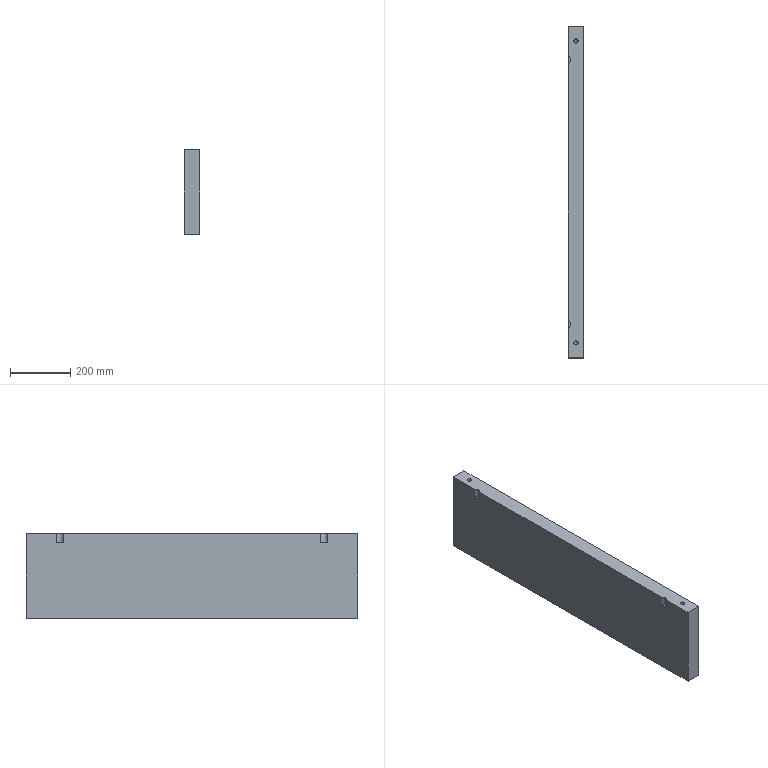Part | NX | features 29 2 | 1 solid | 20 faces | box 50 x 1105 x 280.5 mm | volume 15459680 mm3 | plane 8 | cylinder 7 | cone 5 | commonest cylinder face diameters 14.1 x5 28 x2
STEP:
#1=CARTESIAN_POINT('',(2006.023,-502.5,-493.5));
#2=VERTEX_POINT('',#1);
#3=CARTESIAN_POINT('',(1998.973,-502.5,-493.5));
#4=DIRECTION('',(0.,0.,1.));
#5=DIRECTION('',(1.,0.,0.));
#6=AXIS2_PLACEMENT_3D('',#3,#4,#5);
#7=CIRCLE('',#6,7.05);
#8=EDGE_CURVE('',#2,#2,#7,.T.);
#9=ORIENTED_EDGE('',*,*,#8,.T.);
#10=EDGE_LOOP('',(#9));
#11=FACE_BOUND('',#10,.T.);
#12=CARTESIAN_POINT('',(1973.973,552.5,-493.5));
#13=VERTEX_POINT('',#12);
#14=CARTESIAN_POINT('',(1973.973,-552.5,-493.5));
#15=VERTEX_POINT('',#14);
#16=CARTESIAN_POINT('',(1973.973,193.,-493.5));
#17=DIRECTION('',(0.,-1.,0.));
#18=VECTOR('',#17,1000.);
#19=LINE('',#16,#18);
#20=EDGE_CURVE('',#13,#15,#19,.T.);
#21=ORIENTED_EDGE('',*,*,#20,.F.);
#22=CARTESIAN_POINT('',(2023.973,552.5,-493.5));
#23=VERTEX_POINT('',#22);
#24=CARTESIAN_POINT('',(2773.973,552.5,-493.5));
#25=DIRECTION('',(1.,0.,0.));
#26=VECTOR('',#25,1000.);
#27=LINE('',#24,#26);
#28=EDGE_CURVE('',#13,#23,#27,.T.);
#29=ORIENTED_EDGE('',*,*,#28,.T.);
#30=CARTESIAN_POINT('',(2023.973,-552.5,-493.5));
#31=VERTEX_POINT('',#30);
#32=CARTESIAN_POINT('',(2023.973,193.,-493.5));
#33=DIRECTION('',(0.,1.,0.));
#34=VECTOR('',#33,1000.);
#35=LINE('',#32,#34);
#36=EDGE_CURVE('',#31,#23,#35,.T.);
#37=ORIENTED_EDGE('',*,*,#36,.F.);
#38=CARTESIAN_POINT('',(2773.973,-552.5,-493.5));
#39=DIRECTION('',(-1.,0.,0.));
#40=VECTOR('',#39,1000.);
#41=LINE('',#38,#40);
#42=EDGE_CURVE('',#31,#15,#41,.T.);
#43=ORIENTED_EDGE('',*,*,#42,.T.);
#44=EDGE_LOOP('',(#21,#29,#37,#43));
#45=FACE_BOUND('',#44,.T.);
#46=CARTESIAN_POINT('',(2006.023,502.5,-493.5));
#47=VERTEX_POINT('',#46);
#48=CARTESIAN_POINT('',(1998.973,502.5,-493.5));
#49=DIRECTION('',(0.,0.,1.));
#50=DIRECTION('',(1.,0.,0.));
#51=AXIS2_PLACEMENT_3D('',#48,#49,#50);
#52=CIRCLE('',#51,7.05);
#53=EDGE_CURVE('',#47,#47,#52,.T.);
#54=ORIENTED_EDGE('',*,*,#53,.T.);
#55=EDGE_LOOP('',(#54));
#56=FACE_BOUND('',#55,.T.);
#57=CARTESIAN_POINT('',(2006.023,0.,-493.5));
#58=VERTEX_POINT('',#57);
#59=CARTESIAN_POINT('',(1998.973,0.,-493.5));
#60=DIRECTION('',(0.,0.,1.));
#61=DIRECTION('',(1.,0.,0.));
#62=AXIS2_PLACEMENT_3D('',#59,#60,#61);
#63=CIRCLE('',#62,7.05);
#64=EDGE_CURVE('',#58,#58,#63,.T.);
#65=ORIENTED_EDGE('',*,*,#64,.T.);
#66=EDGE_LOOP('',(#65));
#67=FACE_BOUND('',#66,.T.);
#68=CARTESIAN_POINT('',(2773.973,0.,-493.5));
#69=DIRECTION('',(0.,0.,-1.));
#70=DIRECTION('',(1.,0.,0.));
#71=AXIS2_PLACEMENT_3D('',#68,#69,#70);
#72=PLANE('',#71);
#73=ADVANCED_FACE('',(#11,#45,#56,#67),#72,.T.);
#74=CARTESIAN_POINT('',(2006.023,-502.5,-213.));
#75=VERTEX_POINT('',#74);
#76=CARTESIAN_POINT('',(1998.973,-502.5,-213.));
#77=DIRECTION('',(0.,0.,-1.));
#78=DIRECTION('',(1.,0.,0.));
#79=AXIS2_PLACEMENT_3D('',#76,#77,#78);
#80=CIRCLE('',#79,7.05);
#81=EDGE_CURVE('',#75,#75,#80,.T.);
#82=ORIENTED_EDGE('',*,*,#81,.T.);
#83=EDGE_LOOP('',(#82));
#84=FACE_BOUND('',#83,.T.);
#85=CARTESIAN_POINT('',(1973.973,427.86,-213.));
#86=VERTEX_POINT('',#85);
#87=CARTESIAN_POINT('',(1973.973,452.14,-213.));
#88=VERTEX_POINT('',#87);
#89=CARTESIAN_POINT('',(1967.,440.,-213.));
#90=DIRECTION('',(0.,0.,1.));
#91=DIRECTION('',(-1.,0.,0.));
#92=AXIS2_PLACEMENT_3D('',#89,#90,#91);
#93=CIRCLE('',#92,14.);
#94=EDGE_CURVE('',#86,#88,#93,.T.);
#95=ORIENTED_EDGE('',*,*,#94,.F.);
#96=CARTESIAN_POINT('',(1973.973,-427.86,-213.));
#97=VERTEX_POINT('',#96);
#98=CARTESIAN_POINT('',(1973.973,193.,-213.));
#99=DIRECTION('',(0.,1.,0.));
#100=VECTOR('',#99,1000.);
#101=LINE('',#98,#100);
#102=EDGE_CURVE('',#97,#86,#101,.T.);
#103=ORIENTED_EDGE('',*,*,#102,.F.);
#104=CARTESIAN_POINT('',(1973.973,-452.14,-213.));
#105=VERTEX_POINT('',#104);
#106=CARTESIAN_POINT('',(1967.,-440.,-213.));
#107=DIRECTION('',(0.,0.,-1.));
#108=DIRECTION('',(-1.,0.,0.));
#109=AXIS2_PLACEMENT_3D('',#106,#107,#108);
#110=CIRCLE('',#109,14.);
#111=EDGE_CURVE('',#97,#105,#110,.T.);
#112=ORIENTED_EDGE('',*,*,#111,.T.);
#113=CARTESIAN_POINT('',(1973.973,-552.5,-213.));
#114=VERTEX_POINT('',#113);
#115=CARTESIAN_POINT('',(1973.973,193.,-213.));
#116=DIRECTION('',(0.,1.,0.));
#117=VECTOR('',#116,1000.);
#118=LINE('',#115,#117);
#119=EDGE_CURVE('',#114,#105,#118,.T.);
#120=ORIENTED_EDGE('',*,*,#119,.F.);
#121=CARTESIAN_POINT('',(2023.973,-552.5,-213.));
#122=VERTEX_POINT('',#121);
#123=CARTESIAN_POINT('',(2773.973,-552.5,-213.));
#124=DIRECTION('',(1.,0.,0.));
#125=VECTOR('',#124,1000.);
#126=LINE('',#123,#125);
#127=EDGE_CURVE('',#114,#122,#126,.T.);
#128=ORIENTED_EDGE('',*,*,#127,.T.);
#129=CARTESIAN_POINT('',(2023.973,552.5,-213.));
#130=VERTEX_POINT('',#129);
#131=CARTESIAN_POINT('',(2023.973,193.,-213.));
#132=DIRECTION('',(0.,-1.,0.));
#133=VECTOR('',#132,1000.);
#134=LINE('',#131,#133);
#135=EDGE_CURVE('',#130,#122,#134,.T.);
#136=ORIENTED_EDGE('',*,*,#135,.F.);
#137=CARTESIAN_POINT('',(1973.973,552.5,-213.));
#138=VERTEX_POINT('',#137);
#139=CARTESIAN_POINT('',(2773.973,552.5,-213.));
#140=DIRECTION('',(-1.,0.,0.));
#141=VECTOR('',#140,1000.);
#142=LINE('',#139,#141);
#143=EDGE_CURVE('',#130,#138,#142,.T.);
#144=ORIENTED_EDGE('',*,*,#143,.T.);
#145=CARTESIAN_POINT('',(1973.973,193.,-213.));
#146=DIRECTION('',(0.,1.,0.));
#147=VECTOR('',#146,1000.);
#148=LINE('',#145,#147);
#149=EDGE_CURVE('',#88,#138,#148,.T.);
#150=ORIENTED_EDGE('',*,*,#149,.F.);
#151=EDGE_LOOP('',(#95,#103,#112,#120,#128,#136,#144,#150));
#152=FACE_BOUND('',#151,.T.);
#153=CARTESIAN_POINT('',(2006.023,502.5,-213.));
#154=VERTEX_POINT('',#153);
#155=CARTESIAN_POINT('',(1998.973,502.5,-213.));
#156=DIRECTION('',(0.,0.,-1.));
#157=DIRECTION('',(1.,0.,0.));
#158=AXIS2_PLACEMENT_3D('',#155,#156,#157);
#159=CIRCLE('',#158,7.05);
#160=EDGE_CURVE('',#154,#154,#159,.T.);
#161=ORIENTED_EDGE('',*,*,#160,.T.);
#162=EDGE_LOOP('',(#161));
#163=FACE_BOUND('',#162,.T.);
#164=CARTESIAN_POINT('',(2773.973,0.,-213.));
#165=DIRECTION('',(0.,0.,1.));
#166=DIRECTION('',(-1.,0.,0.));
#167=AXIS2_PLACEMENT_3D('',#164,#165,#166);
#168=PLANE('',#167);
#169=ADVANCED_FACE('',(#84,#152,#163),#168,.T.);
#170=CARTESIAN_POINT('',(1973.973,427.86,-243.));
#171=VERTEX_POINT('',#170);
#172=CARTESIAN_POINT('',(1973.973,427.86,-243.));
#173=DIRECTION('',(0.,0.,1.));
#174=VECTOR('',#173,1000.);
#175=LINE('',#172,#174);
#176=EDGE_CURVE('',#171,#86,#175,.T.);
#177=ORIENTED_EDGE('',*,*,#176,.F.);
#178=CARTESIAN_POINT('',(1973.973,452.14,-243.));
#179=VERTEX_POINT('',#178);
#180=CARTESIAN_POINT('',(1973.973,193.,-243.));
#181=DIRECTION('',(0.,1.,0.));
#182=VECTOR('',#181,1000.);
#183=LINE('',#180,#182);
#184=EDGE_CURVE('',#171,#179,#183,.T.);
#185=ORIENTED_EDGE('',*,*,#184,.T.);
#186=CARTESIAN_POINT('',(1973.973,452.14,-243.));
#187=DIRECTION('',(0.,0.,-1.));
#188=VECTOR('',#187,1000.);
#189=LINE('',#186,#188);
#190=EDGE_CURVE('',#88,#179,#189,.T.);
#191=ORIENTED_EDGE('',*,*,#190,.F.);
#192=ORIENTED_EDGE('',*,*,#149,.T.);
#193=CARTESIAN_POINT('',(1973.973,552.5,-205.5));
#194=DIRECTION('',(0.,0.,-1.));
#195=VECTOR('',#194,1000.);
#196=LINE('',#193,#195);
#197=EDGE_CURVE('',#138,#13,#196,.T.);
#198=ORIENTED_EDGE('',*,*,#197,.T.);
#199=ORIENTED_EDGE('',*,*,#20,.T.);
#200=CARTESIAN_POINT('',(1973.973,-552.5,-205.5));
#201=DIRECTION('',(0.,0.,1.));
#202=VECTOR('',#201,1000.);
#203=LINE('',#200,#202);
#204=EDGE_CURVE('',#15,#114,#203,.T.);
#205=ORIENTED_EDGE('',*,*,#204,.T.);
#206=ORIENTED_EDGE('',*,*,#119,.T.);
#207=CARTESIAN_POINT('',(1973.973,-452.14,-243.));
#208=VERTEX_POINT('',#207);
#209=CARTESIAN_POINT('',(1973.973,-452.14,-243.));
#210=DIRECTION('',(0.,0.,-1.));
#211=VECTOR('',#210,1000.);
#212=LINE('',#209,#211);
#213=EDGE_CURVE('',#105,#208,#212,.T.);
#214=ORIENTED_EDGE('',*,*,#213,.T.);
#215=CARTESIAN_POINT('',(1973.973,-427.86,-243.));
#216=VERTEX_POINT('',#215);
#217=CARTESIAN_POINT('',(1973.973,193.,-243.));
#218=DIRECTION('',(0.,-1.,0.));
#219=VECTOR('',#218,1000.);
#220=LINE('',#217,#219);
#221=EDGE_CURVE('',#216,#208,#220,.T.);
#222=ORIENTED_EDGE('',*,*,#221,.F.);
#223=CARTESIAN_POINT('',(1973.973,-427.86,-243.));
#224=DIRECTION('',(0.,0.,1.));
#225=VECTOR('',#224,1000.);
#226=LINE('',#223,#225);
#227=EDGE_CURVE('',#216,#97,#226,.T.);
#228=ORIENTED_EDGE('',*,*,#227,.T.);
#229=ORIENTED_EDGE('',*,*,#102,.T.);
#230=EDGE_LOOP('',(#177,#185,#191,#192,#198,#199,#205,#206,#214,#222,#228,#229));
#231=FACE_BOUND('',#230,.T.);
#232=CARTESIAN_POINT('',(1973.973,193.,-205.5));
#233=DIRECTION('',(-1.,0.,0.));
#234=DIRECTION('',(0.,0.,1.));
#235=AXIS2_PLACEMENT_3D('',#232,#233,#234);
#236=PLANE('',#235);
#237=ADVANCED_FACE('',(#231),#236,.T.);
#238=ORIENTED_EDGE('',*,*,#143,.F.);
#239=CARTESIAN_POINT('',(2023.973,552.5,-205.5));
#240=DIRECTION('',(0.,0.,1.));
#241=VECTOR('',#240,1000.);
#242=LINE('',#239,#241);
#243=EDGE_CURVE('',#23,#130,#242,.T.);
#244=ORIENTED_EDGE('',*,*,#243,.F.);
#245=ORIENTED_EDGE('',*,*,#28,.F.);
#246=ORIENTED_EDGE('',*,*,#197,.F.);
#247=EDGE_LOOP('',(#238,#244,#245,#246));
#248=FACE_BOUND('',#247,.T.);
#249=CARTESIAN_POINT('',(282.5,552.5,91.));
#250=DIRECTION('',(0.,-1.,0.));
#251=DIRECTION('',(-1.,0.,0.));
#252=AXIS2_PLACEMENT_3D('',#249,#250,#251);
#253=PLANE('',#252);
#254=ADVANCED_FACE('',(#248),#253,.F.);
#255=ORIENTED_EDGE('',*,*,#36,.T.);
#256=ORIENTED_EDGE('',*,*,#243,.T.);
#257=ORIENTED_EDGE('',*,*,#135,.T.);
#258=CARTESIAN_POINT('',(2023.973,-552.5,-205.5));
#259=DIRECTION('',(0.,0.,-1.));
#260=VECTOR('',#259,1000.);
#261=LINE('',#258,#260);
#262=EDGE_CURVE('',#122,#31,#261,.T.);
#263=ORIENTED_EDGE('',*,*,#262,.T.);
#264=EDGE_LOOP('',(#255,#256,#257,#263));
#265=FACE_BOUND('',#264,.T.);
#266=CARTESIAN_POINT('',(2023.973,193.,-205.5));
#267=DIRECTION('',(1.,0.,0.));
#268=DIRECTION('',(0.,0.,-1.));
#269=AXIS2_PLACEMENT_3D('',#266,#267,#268);
#270=PLANE('',#269);
#271=ADVANCED_FACE('',(#265),#270,.T.);
#272=ORIENTED_EDGE('',*,*,#127,.F.);
#273=ORIENTED_EDGE('',*,*,#204,.F.);
#274=ORIENTED_EDGE('',*,*,#42,.F.);
#275=ORIENTED_EDGE('',*,*,#262,.F.);
#276=EDGE_LOOP('',(#272,#273,#274,#275));
#277=FACE_BOUND('',#276,.T.);
#278=CARTESIAN_POINT('',(282.5,-552.5,-113.));
#279=DIRECTION('',(0.,1.,0.));
#280=DIRECTION('',(1.,0.,0.));
#281=AXIS2_PLACEMENT_3D('',#278,#279,#280);
#282=PLANE('',#281);
#283=ADVANCED_FACE('',(#277),#282,.F.);
#284=ORIENTED_EDGE('',*,*,#111,.F.);
#285=ORIENTED_EDGE('',*,*,#227,.F.);
#286=CARTESIAN_POINT('',(1967.,-440.,-243.));
#287=DIRECTION('',(0.,0.,1.));
#288=DIRECTION('',(-1.,0.,0.));
#289=AXIS2_PLACEMENT_3D('',#286,#287,#288);
#290=CIRCLE('',#289,14.);
#291=EDGE_CURVE('',#208,#216,#290,.T.);
#292=ORIENTED_EDGE('',*,*,#291,.F.);
#293=ORIENTED_EDGE('',*,*,#213,.F.);
#294=EDGE_LOOP('',(#284,#285,#292,#293));
#295=FACE_BOUND('',#294,.T.);
#296=CARTESIAN_POINT('',(1967.,-440.,-243.));
#297=DIRECTION('',(0.,0.,1.));
#298=DIRECTION('',(-1.,0.,0.));
#299=AXIS2_PLACEMENT_3D('',#296,#297,#298);
#300=CYLINDRICAL_SURFACE('',#299,14.);
#301=ADVANCED_FACE('',(#295),#300,.F.);
#302=ORIENTED_EDGE('',*,*,#221,.T.);
#303=ORIENTED_EDGE('',*,*,#291,.T.);
#304=EDGE_LOOP('',(#302,#303));
#305=FACE_BOUND('',#304,.T.);
#306=CARTESIAN_POINT('',(1967.,-440.,-243.));
#307=DIRECTION('',(0.,0.,-1.));
#308=DIRECTION('',(1.,0.,0.));
#309=AXIS2_PLACEMENT_3D('',#306,#307,#308);
#310=PLANE('',#309);
#311=ADVANCED_FACE('',(#305),#310,.F.);
#312=ORIENTED_EDGE('',*,*,#176,.T.);
#313=ORIENTED_EDGE('',*,*,#94,.T.);
#314=ORIENTED_EDGE('',*,*,#190,.T.);
#315=CARTESIAN_POINT('',(1967.,440.,-243.));
#316=DIRECTION('',(0.,0.,-1.));
#317=DIRECTION('',(-1.,0.,0.));
#318=AXIS2_PLACEMENT_3D('',#315,#316,#317);
#319=CIRCLE('',#318,14.);
#320=EDGE_CURVE('',#179,#171,#319,.T.);
#321=ORIENTED_EDGE('',*,*,#320,.T.);
#322=EDGE_LOOP('',(#312,#313,#314,#321));
#323=FACE_BOUND('',#322,.T.);
#324=CARTESIAN_POINT('',(1967.,440.,-243.));
#325=DIRECTION('',(0.,0.,1.));
#326=DIRECTION('',(-1.,0.,0.));
#327=AXIS2_PLACEMENT_3D('',#324,#325,#326);
#328=CYLINDRICAL_SURFACE('',#327,14.);
#329=ADVANCED_FACE('',(#323),#328,.F.);
#330=ORIENTED_EDGE('',*,*,#320,.F.);
#331=ORIENTED_EDGE('',*,*,#184,.F.);
#332=EDGE_LOOP('',(#330,#331));
#333=FACE_BOUND('',#332,.T.);
#334=CARTESIAN_POINT('',(1967.,440.,-243.));
#335=DIRECTION('',(0.,0.,1.));
#336=DIRECTION('',(-1.,0.,0.));
#337=AXIS2_PLACEMENT_3D('',#334,#335,#336);
#338=PLANE('',#337);
#339=ADVANCED_FACE('',(#333),#338,.T.);
#340=CARTESIAN_POINT('',(1991.923,-502.5,-249.95));
#341=VERTEX_POINT('',#340);
#342=CARTESIAN_POINT('',(1998.973,-502.5,-249.95));
#343=DIRECTION('',(0.,0.,-1.));
#344=DIRECTION('',(-1.,0.,0.));
#345=AXIS2_PLACEMENT_3D('',#342,#343,#344);
#346=CIRCLE('',#345,7.05);
#347=EDGE_CURVE('',#341,#341,#346,.T.);
#348=ORIENTED_EDGE('',*,*,#347,.T.);
#349=EDGE_LOOP('',(#348));
#350=FACE_BOUND('',#349,.T.);
#351=ORIENTED_EDGE('',*,*,#81,.F.);
#352=EDGE_LOOP('',(#351));
#353=FACE_BOUND('',#352,.T.);
#354=CARTESIAN_POINT('',(1998.973,-502.5,-213.));
#355=DIRECTION('',(0.,0.,-1.));
#356=DIRECTION('',(-1.,0.,0.));
#357=AXIS2_PLACEMENT_3D('',#354,#355,#356);
#358=CYLINDRICAL_SURFACE('',#357,7.05);
#359=ADVANCED_FACE('',(#350,#353),#358,.F.);
#360=CARTESIAN_POINT('',(1998.973,-502.5,-257.));
#361=VERTEX_POINT('',#360);
#362=VERTEX_LOOP('',#361);
#363=FACE_BOUND('',#362,.T.);
#364=ORIENTED_EDGE('',*,*,#347,.F.);
#365=EDGE_LOOP('',(#364));
#366=FACE_BOUND('',#365,.T.);
#367=CARTESIAN_POINT('',(1998.973,-502.5,-249.95));
#368=DIRECTION('',(0.,0.,1.));
#369=DIRECTION('',(-1.,0.,0.));
#370=AXIS2_PLACEMENT_3D('',#367,#368,#369);
#371=CONICAL_SURFACE('',#370,7.05,0.7854);
#372=ADVANCED_FACE('',(#363,#366),#371,.F.);
#373=CARTESIAN_POINT('',(1991.923,502.5,-249.95));
#374=VERTEX_POINT('',#373);
#375=CARTESIAN_POINT('',(1998.973,502.5,-249.95));
#376=DIRECTION('',(0.,0.,-1.));
#377=DIRECTION('',(-1.,0.,0.));
#378=AXIS2_PLACEMENT_3D('',#375,#376,#377);
#379=CIRCLE('',#378,7.05);
#380=EDGE_CURVE('',#374,#374,#379,.T.);
#381=ORIENTED_EDGE('',*,*,#380,.T.);
#382=EDGE_LOOP('',(#381));
#383=FACE_BOUND('',#382,.T.);
#384=ORIENTED_EDGE('',*,*,#160,.F.);
#385=EDGE_LOOP('',(#384));
#386=FACE_BOUND('',#385,.T.);
#387=CARTESIAN_POINT('',(1998.973,502.5,-213.));
#388=DIRECTION('',(0.,0.,-1.));
#389=DIRECTION('',(-1.,0.,0.));
#390=AXIS2_PLACEMENT_3D('',#387,#388,#389);
#391=CYLINDRICAL_SURFACE('',#390,7.05);
#392=ADVANCED_FACE('',(#383,#386),#391,.F.);
#393=CARTESIAN_POINT('',(1998.973,502.5,-257.));
#394=VERTEX_POINT('',#393);
#395=VERTEX_LOOP('',#394);
#396=FACE_BOUND('',#395,.T.);
#397=ORIENTED_EDGE('',*,*,#380,.F.);
#398=EDGE_LOOP('',(#397));
#399=FACE_BOUND('',#398,.T.);
#400=CARTESIAN_POINT('',(1998.973,502.5,-249.95));
#401=DIRECTION('',(0.,0.,1.));
#402=DIRECTION('',(-1.,0.,0.));
#403=AXIS2_PLACEMENT_3D('',#400,#401,#402);
#404=CONICAL_SURFACE('',#403,7.05,0.7854);
#405=ADVANCED_FACE('',(#396,#399),#404,.F.);
#406=CARTESIAN_POINT('',(2006.023,502.5,-456.55));
#407=VERTEX_POINT('',#406);
#408=CARTESIAN_POINT('',(1998.973,502.5,-456.55));
#409=DIRECTION('',(0.,0.,1.));
#410=DIRECTION('',(1.,0.,0.));
#411=AXIS2_PLACEMENT_3D('',#408,#409,#410);
#412=CIRCLE('',#411,7.05);
#413=EDGE_CURVE('',#407,#407,#412,.T.);
#414=ORIENTED_EDGE('',*,*,#413,.T.);
#415=EDGE_LOOP('',(#414));
#416=FACE_BOUND('',#415,.T.);
#417=ORIENTED_EDGE('',*,*,#53,.F.);
#418=EDGE_LOOP('',(#417));
#419=FACE_BOUND('',#418,.T.);
#420=CARTESIAN_POINT('',(1998.973,502.5,-493.5));
#421=DIRECTION('',(0.,0.,1.));
#422=DIRECTION('',(-1.,0.,0.));
#423=AXIS2_PLACEMENT_3D('',#420,#421,#422);
#424=CYLINDRICAL_SURFACE('',#423,7.05);
#425=ADVANCED_FACE('',(#416,#419),#424,.F.);
#426=CARTESIAN_POINT('',(1998.973,502.5,-449.5));
#427=VERTEX_POINT('',#426);
#428=VERTEX_LOOP('',#427);
#429=FACE_BOUND('',#428,.T.);
#430=ORIENTED_EDGE('',*,*,#413,.F.);
#431=EDGE_LOOP('',(#430));
#432=FACE_BOUND('',#431,.T.);
#433=CARTESIAN_POINT('',(1998.973,502.5,-456.55));
#434=DIRECTION('',(0.,0.,-1.));
#435=DIRECTION('',(1.,0.,0.));
#436=AXIS2_PLACEMENT_3D('',#433,#434,#435);
#437=CONICAL_SURFACE('',#436,7.05,0.7854);
#438=ADVANCED_FACE('',(#429,#432),#437,.F.);
#439=CARTESIAN_POINT('',(2006.023,-502.5,-456.55));
#440=VERTEX_POINT('',#439);
#441=CARTESIAN_POINT('',(1998.973,-502.5,-456.55));
#442=DIRECTION('',(0.,0.,1.));
#443=DIRECTION('',(1.,0.,0.));
#444=AXIS2_PLACEMENT_3D('',#441,#442,#443);
#445=CIRCLE('',#444,7.05);
#446=EDGE_CURVE('',#440,#440,#445,.T.);
#447=ORIENTED_EDGE('',*,*,#446,.T.);
#448=EDGE_LOOP('',(#447));
#449=FACE_BOUND('',#448,.T.);
#450=ORIENTED_EDGE('',*,*,#8,.F.);
#451=EDGE_LOOP('',(#450));
#452=FACE_BOUND('',#451,.T.);
#453=CARTESIAN_POINT('',(1998.973,-502.5,-493.5));
#454=DIRECTION('',(0.,0.,1.));
#455=DIRECTION('',(-1.,0.,0.));
#456=AXIS2_PLACEMENT_3D('',#453,#454,#455);
#457=CYLINDRICAL_SURFACE('',#456,7.05);
#458=ADVANCED_FACE('',(#449,#452),#457,.F.);
#459=CARTESIAN_POINT('',(1998.973,-502.5,-449.5));
#460=VERTEX_POINT('',#459);
#461=VERTEX_LOOP('',#460);
#462=FACE_BOUND('',#461,.T.);
#463=ORIENTED_EDGE('',*,*,#446,.F.);
#464=EDGE_LOOP('',(#463));
#465=FACE_BOUND('',#464,.T.);
#466=CARTESIAN_POINT('',(1998.973,-502.5,-456.55));
#467=DIRECTION('',(0.,0.,-1.));
#468=DIRECTION('',(1.,0.,0.));
#469=AXIS2_PLACEMENT_3D('',#466,#467,#468);
#470=CONICAL_SURFACE('',#469,7.05,0.7854);
#471=ADVANCED_FACE('',(#462,#465),#470,.F.);
#472=CARTESIAN_POINT('',(2006.023,0.,-456.55));
#473=VERTEX_POINT('',#472);
#474=CARTESIAN_POINT('',(1998.973,0.,-456.55));
#475=DIRECTION('',(0.,0.,1.));
#476=DIRECTION('',(1.,0.,0.));
#477=AXIS2_PLACEMENT_3D('',#474,#475,#476);
#478=CIRCLE('',#477,7.05);
#479=EDGE_CURVE('',#473,#473,#478,.T.);
#480=ORIENTED_EDGE('',*,*,#479,.T.);
#481=EDGE_LOOP('',(#480));
#482=FACE_BOUND('',#481,.T.);
#483=ORIENTED_EDGE('',*,*,#64,.F.);
#484=EDGE_LOOP('',(#483));
#485=FACE_BOUND('',#484,.T.);
#486=CARTESIAN_POINT('',(1998.973,0.,-493.5));
#487=DIRECTION('',(0.,0.,1.));
#488=DIRECTION('',(-1.,0.,0.));
#489=AXIS2_PLACEMENT_3D('',#486,#487,#488);
#490=CYLINDRICAL_SURFACE('',#489,7.05);
#491=ADVANCED_FACE('',(#482,#485),#490,.F.);
#492=CARTESIAN_POINT('',(1998.973,0.,-449.5));
#493=VERTEX_POINT('',#492);
#494=VERTEX_LOOP('',#493);
#495=FACE_BOUND('',#494,.T.);
#496=ORIENTED_EDGE('',*,*,#479,.F.);
#497=EDGE_LOOP('',(#496));
#498=FACE_BOUND('',#497,.T.);
#499=CARTESIAN_POINT('',(1998.973,0.,-456.55));
#500=DIRECTION('',(0.,0.,-1.));
#501=DIRECTION('',(1.,0.,0.));
#502=AXIS2_PLACEMENT_3D('',#499,#500,#501);
#503=CONICAL_SURFACE('',#502,7.05,0.7854);
#504=ADVANCED_FACE('',(#495,#498),#503,.F.);
#505=CLOSED_SHELL('',(#73,#169,#237,#254,#271,#283,#301,#311,#329,#339,#359,#372,#392,#405,#425,#438,#458,#471,#491,#504));
#506=MANIFOLD_SOLID_BREP('',#505);
#507=(LENGTH_UNIT()NAMED_UNIT(*)SI_UNIT(.MILLI.,.METRE.));
#508=UNCERTAINTY_MEASURE_WITH_UNIT(LENGTH_MEASURE(0.00001),#507,'','');
#509=(NAMED_UNIT(*)PLANE_ANGLE_UNIT()SI_UNIT($,.RADIAN.));
#510=(NAMED_UNIT(*)SI_UNIT($,.STERADIAN.)SOLID_ANGLE_UNIT());
#511=(GEOMETRIC_REPRESENTATION_CONTEXT(3)GLOBAL_UNCERTAINTY_ASSIGNED_CONTEXT((#508))GLOBAL_UNIT_ASSIGNED_CONTEXT((#507,#509,#510))REPRESENTATION_CONTEXT('',''));
#512=ADVANCED_BREP_SHAPE_REPRESENTATION('',(#506),#511);